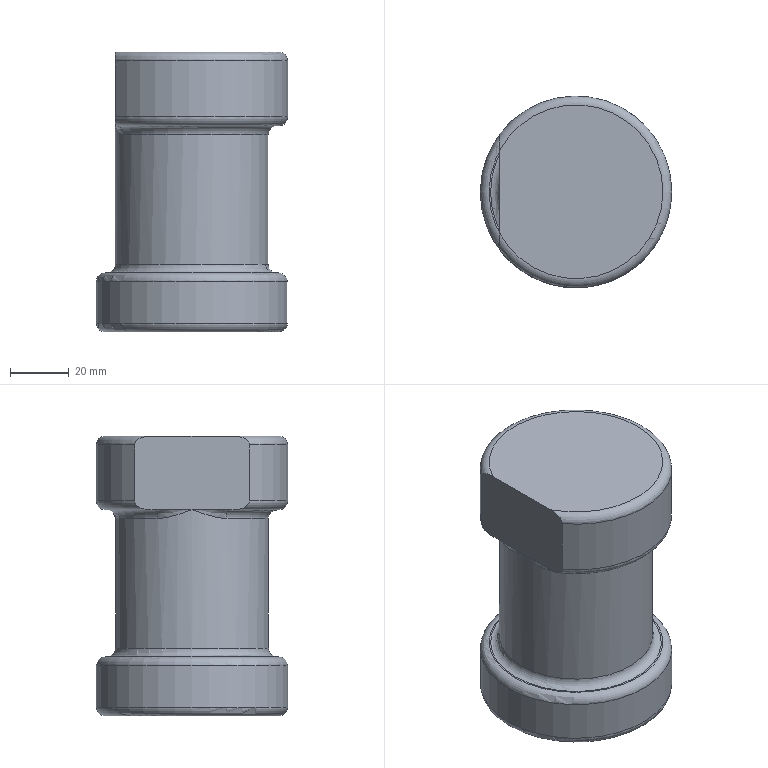Part | NX | features solid 2 | 1 solid | 19 faces | box 65 x 65 x 95 mm | volume 199108 mm3 | torus 6 | plane 5 | cylinder 4 | cone 2 | spline 2 | commonest cylinder face diameters 65 x2 28 x1 52 x1
STEP:
#1=CARTESIAN_POINT('',(-546.,345.5,87.));
#2=VERTEX_POINT('',#1);
#3=CARTESIAN_POINT('',(-546.,345.5,68.));
#4=VERTEX_POINT('',#3);
#5=CARTESIAN_POINT('',(-546.,345.5,90.));
#6=DIRECTION('',(0.,0.,-1.));
#7=VECTOR('',#6,1000.);
#8=LINE('',#5,#7);
#9=EDGE_CURVE('',#2,#4,#8,.T.);
#10=ORIENTED_EDGE('',*,*,#9,.T.);
#11=CARTESIAN_POINT('',(-546.,384.5,68.));
#12=VERTEX_POINT('',#11);
#13=CARTESIAN_POINT('',(-520.,365.,68.));
#14=DIRECTION('',(0.,0.,-1.));
#15=DIRECTION('',(-1.,0.,0.));
#16=AXIS2_PLACEMENT_3D('',#13,#14,#15);
#17=CIRCLE('',#16,32.5);
#18=EDGE_CURVE('',#4,#12,#17,.F.);
#19=ORIENTED_EDGE('',*,*,#18,.T.);
#20=CARTESIAN_POINT('',(-546.,384.5,87.));
#21=VERTEX_POINT('',#20);
#22=CARTESIAN_POINT('',(-546.,384.5,90.));
#23=DIRECTION('',(0.,0.,-1.));
#24=VECTOR('',#23,1000.);
#25=LINE('',#22,#24);
#26=EDGE_CURVE('',#12,#21,#25,.F.);
#27=ORIENTED_EDGE('',*,*,#26,.T.);
#28=CARTESIAN_POINT('',(-520.,365.,87.));
#29=DIRECTION('',(0.,0.,-1.));
#30=DIRECTION('',(-1.,0.,0.));
#31=AXIS2_PLACEMENT_3D('',#28,#29,#30);
#32=CIRCLE('',#31,32.5);
#33=EDGE_CURVE('',#21,#2,#32,.T.);
#34=ORIENTED_EDGE('',*,*,#33,.T.);
#35=EDGE_LOOP('',(#10,#19,#27,#34));
#36=FACE_BOUND('',#35,.T.);
#37=CARTESIAN_POINT('',(-520.,365.,-5.));
#38=DIRECTION('',(0.,0.,1.));
#39=DIRECTION('',(1.,0.,0.));
#40=AXIS2_PLACEMENT_3D('',#37,#38,#39);
#41=CYLINDRICAL_SURFACE('',#40,32.5);
#42=ADVANCED_FACE('',(#36),#41,.T.);
#43=CARTESIAN_POINT('',(-546.,351.063,90.));
#44=VERTEX_POINT('',#43);
#45=CARTESIAN_POINT('',(-546.,378.937,90.));
#46=VERTEX_POINT('',#45);
#47=CARTESIAN_POINT('',(-546.,345.5,90.));
#48=DIRECTION('',(0.,1.,0.));
#49=VECTOR('',#48,1000.);
#50=LINE('',#47,#49);
#51=EDGE_CURVE('',#44,#46,#50,.T.);
#52=ORIENTED_EDGE('',*,*,#51,.F.);
#53=CARTESIAN_POINT('',(-520.,365.,90.));
#54=DIRECTION('',(0.,0.,-1.));
#55=DIRECTION('',(-1.,0.,0.));
#56=AXIS2_PLACEMENT_3D('',#53,#54,#55);
#57=CIRCLE('',#56,29.5);
#58=EDGE_CURVE('',#44,#46,#57,.F.);
#59=ORIENTED_EDGE('',*,*,#58,.T.);
#60=EDGE_LOOP('',(#52,#59));
#61=FACE_BOUND('',#60,.T.);
#62=CARTESIAN_POINT('',(-520.,365.,90.));
#63=DIRECTION('',(0.,0.,-1.));
#64=DIRECTION('',(-1.,0.,0.));
#65=AXIS2_PLACEMENT_3D('',#62,#63,#64);
#66=PLANE('',#65);
#67=ADVANCED_FACE('',(#61),#66,.F.);
#68=CARTESIAN_POINT('',(-546.,351.063,65.));
#69=VERTEX_POINT('',#68);
#70=CARTESIAN_POINT('',(-546.,352.155,65.));
#71=VERTEX_POINT('',#70);
#72=CARTESIAN_POINT('',(-546.,365.,65.));
#73=DIRECTION('',(0.,1.,0.));
#74=VECTOR('',#73,1000.);
#75=LINE('',#72,#74);
#76=EDGE_CURVE('',#69,#71,#75,.T.);
#77=ORIENTED_EDGE('',*,*,#76,.T.);
#78=CARTESIAN_POINT('',(-546.,377.845,65.));
#79=VERTEX_POINT('',#78);
#80=CARTESIAN_POINT('',(-520.,365.,65.));
#81=DIRECTION('',(0.,0.,-1.));
#82=DIRECTION('',(-1.,0.,0.));
#83=AXIS2_PLACEMENT_3D('',#80,#81,#82);
#84=CIRCLE('',#83,29.);
#85=EDGE_CURVE('',#71,#79,#84,.F.);
#86=ORIENTED_EDGE('',*,*,#85,.T.);
#87=CARTESIAN_POINT('',(-546.,378.937,65.));
#88=VERTEX_POINT('',#87);
#89=CARTESIAN_POINT('',(-546.,365.,65.));
#90=DIRECTION('',(0.,1.,0.));
#91=VECTOR('',#90,1000.);
#92=LINE('',#89,#91);
#93=EDGE_CURVE('',#79,#88,#92,.T.);
#94=ORIENTED_EDGE('',*,*,#93,.T.);
#95=CARTESIAN_POINT('',(-520.,365.,65.));
#96=DIRECTION('',(0.,0.,-1.));
#97=DIRECTION('',(-1.,0.,0.));
#98=AXIS2_PLACEMENT_3D('',#95,#96,#97);
#99=CIRCLE('',#98,29.5);
#100=EDGE_CURVE('',#88,#69,#99,.T.);
#101=ORIENTED_EDGE('',*,*,#100,.T.);
#102=EDGE_LOOP('',(#77,#86,#94,#101));
#103=FACE_BOUND('',#102,.T.);
#104=CARTESIAN_POINT('',(-520.,365.,65.));
#105=DIRECTION('',(0.,0.,-1.));
#106=DIRECTION('',(-1.,0.,0.));
#107=AXIS2_PLACEMENT_3D('',#104,#105,#106);
#108=PLANE('',#107);
#109=ADVANCED_FACE('',(#103),#108,.T.);
#110=ORIENTED_EDGE('',*,*,#58,.F.);
#111=CARTESIAN_POINT('',(-546.,351.063,90.));
#112=CARTESIAN_POINT('',(-546.,349.918,90.));
#113=CARTESIAN_POINT('',(-546.,348.171,89.797));
#114=CARTESIAN_POINT('',(-546.,346.107,88.666));
#115=CARTESIAN_POINT('',(-546.,345.5,87.58));
#116=CARTESIAN_POINT('',(-546.,345.5,87.));
#117=B_SPLINE_CURVE_WITH_KNOTS('',3,(#111,#112,#113,#114,#115,#116),.UNSPECIFIED.,.F.,.F.,(4,1,1,4),(0.02888,0.03234,0.03407,0.03579),.UNSPECIFIED.);
#118=EDGE_CURVE('',#44,#2,#117,.T.);
#119=ORIENTED_EDGE('',*,*,#118,.T.);
#120=ORIENTED_EDGE('',*,*,#33,.F.);
#121=CARTESIAN_POINT('',(-546.,384.5,87.));
#122=CARTESIAN_POINT('',(-546.,384.5,87.578));
#123=CARTESIAN_POINT('',(-546.,383.893,88.668));
#124=CARTESIAN_POINT('',(-546.,381.825,89.797));
#125=CARTESIAN_POINT('',(-546.,380.08,90.));
#126=CARTESIAN_POINT('',(-546.,378.937,90.));
#127=B_SPLINE_CURVE_WITH_KNOTS('',3,(#121,#122,#123,#124,#125,#126),.UNSPECIFIED.,.F.,.F.,(4,1,1,4),(0.01647,0.0182,0.01994,0.02342),.UNSPECIFIED.);
#128=EDGE_CURVE('',#21,#46,#127,.T.);
#129=ORIENTED_EDGE('',*,*,#128,.T.);
#130=EDGE_LOOP('',(#110,#119,#120,#129));
#131=FACE_BOUND('',#130,.T.);
#132=CARTESIAN_POINT('',(-520.,365.,87.));
#133=DIRECTION('',(0.,0.,-1.));
#134=DIRECTION('',(-1.,0.,0.));
#135=AXIS2_PLACEMENT_3D('',#132,#133,#134);
#136=TOROIDAL_SURFACE('',#135,29.5,3.);
#137=ADVANCED_FACE('',(#131),#136,.T.);
#138=CARTESIAN_POINT('',(-549.,365.,15.));
#139=VERTEX_POINT('',#138);
#140=CARTESIAN_POINT('',(-520.,365.,15.));
#141=DIRECTION('',(0.,0.,-1.));
#142=DIRECTION('',(-1.,0.,0.));
#143=AXIS2_PLACEMENT_3D('',#140,#141,#142);
#144=CIRCLE('',#143,29.);
#145=EDGE_CURVE('',#139,#139,#144,.T.);
#146=ORIENTED_EDGE('',*,*,#145,.T.);
#147=EDGE_LOOP('',(#146));
#148=FACE_BOUND('',#147,.T.);
#149=CARTESIAN_POINT('',(-549.5,365.,15.));
#150=VERTEX_POINT('',#149);
#151=CARTESIAN_POINT('',(-520.,365.,15.));
#152=DIRECTION('',(0.,0.,-1.));
#153=DIRECTION('',(-1.,0.,0.));
#154=AXIS2_PLACEMENT_3D('',#151,#152,#153);
#155=CIRCLE('',#154,29.5);
#156=EDGE_CURVE('',#150,#150,#155,.F.);
#157=ORIENTED_EDGE('',*,*,#156,.T.);
#158=EDGE_LOOP('',(#157));
#159=FACE_BOUND('',#158,.T.);
#160=CARTESIAN_POINT('',(-520.,365.,15.));
#161=DIRECTION('',(0.,0.,-1.));
#162=DIRECTION('',(-1.,0.,0.));
#163=AXIS2_PLACEMENT_3D('',#160,#161,#162);
#164=PLANE('',#163);
#165=ADVANCED_FACE('',(#148,#159),#164,.F.);
#166=CARTESIAN_POINT('',(-546.,365.,18.));
#167=VERTEX_POINT('',#166);
#168=CARTESIAN_POINT('',(-520.,365.,18.));
#169=DIRECTION('',(0.,0.,-1.));
#170=DIRECTION('',(-1.,0.,0.));
#171=AXIS2_PLACEMENT_3D('',#168,#169,#170);
#172=CIRCLE('',#171,26.);
#173=EDGE_CURVE('',#167,#167,#172,.F.);
#174=ORIENTED_EDGE('',*,*,#173,.T.);
#175=EDGE_LOOP('',(#174));
#176=FACE_BOUND('',#175,.T.);
#177=CARTESIAN_POINT('',(-543.31,353.484,62.));
#178=VERTEX_POINT('',#177);
#179=CARTESIAN_POINT('',(-546.,365.,65.));
#180=VERTEX_POINT('',#179);
#181=CARTESIAN_POINT('',(-543.31,353.484,62.));
#182=CARTESIAN_POINT('',(-544.233,355.351,62.));
#183=CARTESIAN_POINT('',(-545.571,359.193,62.924));
#184=CARTESIAN_POINT('',(-546.,363.039,64.297));
#185=CARTESIAN_POINT('',(-546.,365.,65.));
#186=B_SPLINE_CURVE_WITH_KNOTS('',3,(#181,#182,#183,#184,#185),.UNSPECIFIED.,.F.,.F.,(4,1,4),(0.,0.006249,0.0125),.UNSPECIFIED.);
#187=EDGE_CURVE('',#178,#180,#186,.T.);
#188=ORIENTED_EDGE('',*,*,#187,.T.);
#189=CARTESIAN_POINT('',(-543.31,376.516,62.));
#190=VERTEX_POINT('',#189);
#191=CARTESIAN_POINT('',(-543.31,376.516,62.));
#192=CARTESIAN_POINT('',(-544.233,374.649,62.));
#193=CARTESIAN_POINT('',(-545.571,370.807,62.924));
#194=CARTESIAN_POINT('',(-546.,366.961,64.297));
#195=CARTESIAN_POINT('',(-546.,365.,65.));
#196=B_SPLINE_CURVE_WITH_KNOTS('',3,(#191,#192,#193,#194,#195),.UNSPECIFIED.,.F.,.F.,(4,1,4),(0.,0.006249,0.0125),.UNSPECIFIED.);
#197=EDGE_CURVE('',#180,#190,#196,.F.);
#198=ORIENTED_EDGE('',*,*,#197,.T.);
#199=CARTESIAN_POINT('',(-520.,365.,62.));
#200=DIRECTION('',(0.,0.,-1.));
#201=DIRECTION('',(-1.,0.,0.));
#202=AXIS2_PLACEMENT_3D('',#199,#200,#201);
#203=CIRCLE('',#202,26.);
#204=EDGE_CURVE('',#190,#178,#203,.T.);
#205=ORIENTED_EDGE('',*,*,#204,.T.);
#206=EDGE_LOOP('',(#188,#198,#205));
#207=FACE_BOUND('',#206,.T.);
#208=CARTESIAN_POINT('',(-520.,365.,40.));
#209=DIRECTION('',(0.,0.,-1.));
#210=DIRECTION('',(-1.,0.,0.));
#211=AXIS2_PLACEMENT_3D('',#208,#209,#210);
#212=CYLINDRICAL_SURFACE('',#211,26.);
#213=ADVANCED_FACE('',(#176,#207),#212,.T.);
#214=CARTESIAN_POINT('',(-549.5,365.,-5.));
#215=VERTEX_POINT('',#214);
#216=CARTESIAN_POINT('',(-520.,365.,-5.));
#217=DIRECTION('',(0.,0.,-1.));
#218=DIRECTION('',(-1.,0.,0.));
#219=AXIS2_PLACEMENT_3D('',#216,#217,#218);
#220=CIRCLE('',#219,29.5);
#221=EDGE_CURVE('',#215,#215,#220,.T.);
#222=ORIENTED_EDGE('',*,*,#221,.T.);
#223=EDGE_LOOP('',(#222));
#224=FACE_BOUND('',#223,.T.);
#225=CARTESIAN_POINT('',(-499.,365.,-5.));
#226=VERTEX_POINT('',#225);
#227=CARTESIAN_POINT('',(-520.,365.,-5.));
#228=DIRECTION('',(0.,0.,1.));
#229=DIRECTION('',(1.,0.,0.));
#230=AXIS2_PLACEMENT_3D('',#227,#228,#229);
#231=CIRCLE('',#230,21.);
#232=EDGE_CURVE('',#226,#226,#231,.T.);
#233=ORIENTED_EDGE('',*,*,#232,.T.);
#234=EDGE_LOOP('',(#233));
#235=FACE_BOUND('',#234,.T.);
#236=CARTESIAN_POINT('',(-520.,365.,-5.));
#237=DIRECTION('',(0.,0.,-1.));
#238=DIRECTION('',(-1.,0.,0.));
#239=AXIS2_PLACEMENT_3D('',#236,#237,#238);
#240=PLANE('',#239);
#241=ADVANCED_FACE('',(#224,#235),#240,.T.);
#242=CARTESIAN_POINT('',(-552.5,365.,-2.));
#243=VERTEX_POINT('',#242);
#244=CARTESIAN_POINT('',(-520.,365.,-2.));
#245=DIRECTION('',(0.,0.,-1.));
#246=DIRECTION('',(-1.,0.,0.));
#247=AXIS2_PLACEMENT_3D('',#244,#245,#246);
#248=CIRCLE('',#247,32.5);
#249=EDGE_CURVE('',#243,#243,#248,.F.);
#250=ORIENTED_EDGE('',*,*,#249,.T.);
#251=EDGE_LOOP('',(#250));
#252=FACE_BOUND('',#251,.T.);
#253=CARTESIAN_POINT('',(-552.5,365.,12.));
#254=VERTEX_POINT('',#253);
#255=CARTESIAN_POINT('',(-520.,365.,12.));
#256=DIRECTION('',(0.,0.,-1.));
#257=DIRECTION('',(-1.,0.,0.));
#258=AXIS2_PLACEMENT_3D('',#255,#256,#257);
#259=CIRCLE('',#258,32.5);
#260=EDGE_CURVE('',#254,#254,#259,.T.);
#261=ORIENTED_EDGE('',*,*,#260,.T.);
#262=EDGE_LOOP('',(#261));
#263=FACE_BOUND('',#262,.T.);
#264=CARTESIAN_POINT('',(-520.,365.,-5.));
#265=DIRECTION('',(0.,0.,1.));
#266=DIRECTION('',(1.,0.,0.));
#267=AXIS2_PLACEMENT_3D('',#264,#265,#266);
#268=CYLINDRICAL_SURFACE('',#267,32.5);
#269=ADVANCED_FACE('',(#252,#263),#268,.T.);
#270=CARTESIAN_POINT('',(-506.,365.,70.));
#271=VERTEX_POINT('',#270);
#272=CARTESIAN_POINT('',(-520.,365.,70.));
#273=DIRECTION('',(0.,0.,1.));
#274=DIRECTION('',(1.,0.,0.));
#275=AXIS2_PLACEMENT_3D('',#272,#273,#274);
#276=CIRCLE('',#275,14.);
#277=EDGE_CURVE('',#271,#271,#276,.T.);
#278=ORIENTED_EDGE('',*,*,#277,.F.);
#279=EDGE_LOOP('',(#278));
#280=FACE_BOUND('',#279,.T.);
#281=CARTESIAN_POINT('',(-520.,365.,73.751));
#282=VERTEX_POINT('',#281);
#283=VERTEX_LOOP('',#282);
#284=FACE_BOUND('',#283,.T.);
#285=CARTESIAN_POINT('',(-520.,365.,70.));
#286=DIRECTION('',(0.,0.,-1.));
#287=DIRECTION('',(-1.,0.,0.));
#288=AXIS2_PLACEMENT_3D('',#285,#286,#287);
#289=CONICAL_SURFACE('',#288,14.,1.309);
#290=ADVANCED_FACE('',(#280,#284),#289,.F.);
#291=ORIENTED_EDGE('',*,*,#277,.T.);
#292=EDGE_LOOP('',(#291));
#293=FACE_BOUND('',#292,.T.);
#294=CARTESIAN_POINT('',(-506.,365.,7.124));
#295=VERTEX_POINT('',#294);
#296=CARTESIAN_POINT('',(-520.,365.,7.124));
#297=DIRECTION('',(0.,0.,1.));
#298=DIRECTION('',(1.,0.,0.));
#299=AXIS2_PLACEMENT_3D('',#296,#297,#298);
#300=CIRCLE('',#299,14.);
#301=EDGE_CURVE('',#295,#295,#300,.T.);
#302=ORIENTED_EDGE('',*,*,#301,.F.);
#303=EDGE_LOOP('',(#302));
#304=FACE_BOUND('',#303,.T.);
#305=CARTESIAN_POINT('',(-520.,365.,70.));
#306=DIRECTION('',(0.,0.,1.));
#307=DIRECTION('',(1.,0.,0.));
#308=AXIS2_PLACEMENT_3D('',#305,#306,#307);
#309=CYLINDRICAL_SURFACE('',#308,14.);
#310=ADVANCED_FACE('',(#293,#304),#309,.F.);
#311=ORIENTED_EDGE('',*,*,#301,.T.);
#312=EDGE_LOOP('',(#311));
#313=FACE_BOUND('',#312,.T.);
#314=ORIENTED_EDGE('',*,*,#232,.F.);
#315=EDGE_LOOP('',(#314));
#316=FACE_BOUND('',#315,.T.);
#317=CARTESIAN_POINT('',(-520.,365.,-5.));
#318=DIRECTION('',(0.,0.,-1.));
#319=DIRECTION('',(-1.,0.,0.));
#320=AXIS2_PLACEMENT_3D('',#317,#318,#319);
#321=CONICAL_SURFACE('',#320,21.,0.5236);
#322=ADVANCED_FACE('',(#313,#316),#321,.F.);
#323=ORIENTED_EDGE('',*,*,#76,.F.);
#324=CARTESIAN_POINT('',(-546.,351.063,65.));
#325=CARTESIAN_POINT('',(-546.,349.908,65.));
#326=CARTESIAN_POINT('',(-546.,348.177,65.202));
#327=CARTESIAN_POINT('',(-546.,346.108,66.334));
#328=CARTESIAN_POINT('',(-546.,345.5,67.414));
#329=CARTESIAN_POINT('',(-546.,345.5,68.));
#330=B_SPLINE_CURVE_WITH_KNOTS('',3,(#324,#325,#326,#327,#328,#329),.UNSPECIFIED.,.F.,.F.,(4,1,1,4),(0.,0.003431,0.005146,0.006862),.UNSPECIFIED.);
#331=EDGE_CURVE('',#69,#4,#330,.T.);
#332=ORIENTED_EDGE('',*,*,#331,.T.);
#333=ORIENTED_EDGE('',*,*,#9,.F.);
#334=ORIENTED_EDGE('',*,*,#118,.F.);
#335=ORIENTED_EDGE('',*,*,#51,.T.);
#336=ORIENTED_EDGE('',*,*,#128,.F.);
#337=ORIENTED_EDGE('',*,*,#26,.F.);
#338=CARTESIAN_POINT('',(-546.,384.5,68.));
#339=CARTESIAN_POINT('',(-546.,384.5,67.413));
#340=CARTESIAN_POINT('',(-546.,383.893,66.337));
#341=CARTESIAN_POINT('',(-546.,381.832,65.204));
#342=CARTESIAN_POINT('',(-546.,380.093,65.));
#343=CARTESIAN_POINT('',(-546.,378.937,65.));
#344=B_SPLINE_CURVE_WITH_KNOTS('',3,(#338,#339,#340,#341,#342,#343),.UNSPECIFIED.,.F.,.F.,(4,1,1,4),(0.,0.001726,0.003452,0.006904),.UNSPECIFIED.);
#345=EDGE_CURVE('',#12,#88,#344,.T.);
#346=ORIENTED_EDGE('',*,*,#345,.T.);
#347=ORIENTED_EDGE('',*,*,#93,.F.);
#348=CARTESIAN_POINT('',(-546.,365.,65.));
#349=DIRECTION('',(0.,1.,0.));
#350=VECTOR('',#349,1000.);
#351=LINE('',#348,#350);
#352=EDGE_CURVE('',#180,#79,#351,.T.);
#353=ORIENTED_EDGE('',*,*,#352,.F.);
#354=CARTESIAN_POINT('',(-546.,365.,65.));
#355=DIRECTION('',(0.,1.,0.));
#356=VECTOR('',#355,1000.);
#357=LINE('',#354,#356);
#358=EDGE_CURVE('',#71,#180,#357,.T.);
#359=ORIENTED_EDGE('',*,*,#358,.F.);
#360=EDGE_LOOP('',(#323,#332,#333,#334,#335,#336,#337,#346,#347,#353,#359));
#361=FACE_BOUND('',#360,.T.);
#362=CARTESIAN_POINT('',(-546.,345.5,90.));
#363=DIRECTION('',(-1.,0.,0.));
#364=DIRECTION('',(0.,0.,1.));
#365=AXIS2_PLACEMENT_3D('',#362,#363,#364);
#366=PLANE('',#365);
#367=ADVANCED_FACE('',(#361),#366,.T.);
#368=ORIENTED_EDGE('',*,*,#249,.F.);
#369=EDGE_LOOP('',(#368));
#370=FACE_BOUND('',#369,.T.);
#371=ORIENTED_EDGE('',*,*,#221,.F.);
#372=EDGE_LOOP('',(#371));
#373=FACE_BOUND('',#372,.T.);
#374=CARTESIAN_POINT('',(-520.,365.,-2.));
#375=DIRECTION('',(0.,0.,-1.));
#376=DIRECTION('',(-1.,0.,0.));
#377=AXIS2_PLACEMENT_3D('',#374,#375,#376);
#378=TOROIDAL_SURFACE('',#377,29.5,3.);
#379=ADVANCED_FACE('',(#370,#373),#378,.T.);
#380=ORIENTED_EDGE('',*,*,#358,.T.);
#381=ORIENTED_EDGE('',*,*,#187,.F.);
#382=CARTESIAN_POINT('',(-546.,352.155,62.));
#383=DIRECTION('',(0.4429,-0.8966,0.));
#384=DIRECTION('',(-0.8966,-0.4429,0.));
#385=AXIS2_PLACEMENT_3D('',#382,#383,#384);
#386=CIRCLE('',#385,3.);
#387=EDGE_CURVE('',#71,#178,#386,.F.);
#388=ORIENTED_EDGE('',*,*,#387,.F.);
#389=EDGE_LOOP('',(#380,#381,#388));
#390=FACE_BOUND('',#389,.T.);
#391=CARTESIAN_POINT('',(-543.31,353.484,62.));
#392=CARTESIAN_POINT('',(-543.31,353.484,65.));
#393=CARTESIAN_POINT('',(-546.,352.155,65.));
#394=CARTESIAN_POINT('',(-543.767,354.407,62.));
#395=CARTESIAN_POINT('',(-543.642,354.154,64.576));
#396=CARTESIAN_POINT('',(-546.,353.185,65.));
#397=CARTESIAN_POINT('',(-544.558,356.284,62.245));
#398=CARTESIAN_POINT('',(-544.393,355.827,64.102));
#399=CARTESIAN_POINT('',(-546.,355.278,65.));
#400=CARTESIAN_POINT('',(-545.676,360.138,63.248));
#401=CARTESIAN_POINT('',(-545.587,359.67,64.099));
#402=CARTESIAN_POINT('',(-546.,359.577,65.));
#403=CARTESIAN_POINT('',(-546.,363.037,64.296));
#404=CARTESIAN_POINT('',(-546.,362.924,64.648));
#405=CARTESIAN_POINT('',(-546.,362.811,65.));
#406=CARTESIAN_POINT('',(-546.,365.,65.));
#407=CARTESIAN_POINT('',(-546.,365.,65.));
#408=CARTESIAN_POINT('',(-546.,365.,65.));
#409=(BOUNDED_SURFACE()B_SPLINE_SURFACE(3,2,((#391,#392,#393),(#394,#395,#396),(#397,#398,#399),(#400,#401,#402),(#403,#404,#405),(#406,#407,#408)),.UNSPECIFIED.,.F.,.F.,.F.)B_SPLINE_SURFACE_WITH_KNOTS((4,1,1,4),(3,3),(0.00704,0.01049,0.01394,0.02084),(0.,1.),.UNSPECIFIED.)GEOMETRIC_REPRESENTATION_ITEM()RATIONAL_B_SPLINE_SURFACE(((1.,0.7071,1.),(1.,0.7609,1.),(1.,0.8488,1.),(1.,0.9673,1.),(1.,1.,1.),(1.,1.,1.)))REPRESENTATION_ITEM('')SURFACE());
#410=ADVANCED_FACE('',(#390),#409,.F.);
#411=ORIENTED_EDGE('',*,*,#387,.T.);
#412=ORIENTED_EDGE('',*,*,#204,.F.);
#413=CARTESIAN_POINT('',(-546.,377.845,62.));
#414=DIRECTION('',(0.4429,0.8966,0.));
#415=DIRECTION('',(0.8966,-0.4429,0.));
#416=AXIS2_PLACEMENT_3D('',#413,#414,#415);
#417=CIRCLE('',#416,3.);
#418=EDGE_CURVE('',#79,#190,#417,.T.);
#419=ORIENTED_EDGE('',*,*,#418,.F.);
#420=ORIENTED_EDGE('',*,*,#85,.F.);
#421=EDGE_LOOP('',(#411,#412,#419,#420));
#422=FACE_BOUND('',#421,.T.);
#423=CARTESIAN_POINT('',(-520.,365.,62.));
#424=DIRECTION('',(0.,0.,-1.));
#425=DIRECTION('',(-1.,0.,0.));
#426=AXIS2_PLACEMENT_3D('',#423,#424,#425);
#427=TOROIDAL_SURFACE('',#426,29.,3.);
#428=ADVANCED_FACE('',(#422),#427,.F.);
#429=ORIENTED_EDGE('',*,*,#197,.F.);
#430=ORIENTED_EDGE('',*,*,#352,.T.);
#431=ORIENTED_EDGE('',*,*,#418,.T.);
#432=EDGE_LOOP('',(#429,#430,#431));
#433=FACE_BOUND('',#432,.T.);
#434=CARTESIAN_POINT('',(-546.,377.845,65.));
#435=CARTESIAN_POINT('',(-543.31,376.516,65.));
#436=CARTESIAN_POINT('',(-543.31,376.516,62.));
#437=CARTESIAN_POINT('',(-546.,376.815,65.));
#438=CARTESIAN_POINT('',(-543.642,375.846,64.576));
#439=CARTESIAN_POINT('',(-543.767,375.593,62.));
#440=CARTESIAN_POINT('',(-546.,374.722,65.));
#441=CARTESIAN_POINT('',(-544.393,374.173,64.102));
#442=CARTESIAN_POINT('',(-544.558,373.716,62.245));
#443=CARTESIAN_POINT('',(-546.,370.423,65.));
#444=CARTESIAN_POINT('',(-545.587,370.33,64.099));
#445=CARTESIAN_POINT('',(-545.676,369.862,63.248));
#446=CARTESIAN_POINT('',(-546.,367.189,65.));
#447=CARTESIAN_POINT('',(-546.,367.076,64.648));
#448=CARTESIAN_POINT('',(-546.,366.963,64.296));
#449=CARTESIAN_POINT('',(-546.,365.,65.));
#450=CARTESIAN_POINT('',(-546.,365.,65.));
#451=CARTESIAN_POINT('',(-546.,365.,65.));
#452=(BOUNDED_SURFACE()B_SPLINE_SURFACE(3,2,((#434,#435,#436),(#437,#438,#439),(#440,#441,#442),(#443,#444,#445),(#446,#447,#448),(#449,#450,#451)),.UNSPECIFIED.,.F.,.F.,.F.)B_SPLINE_SURFACE_WITH_KNOTS((4,1,1,4),(3,3),(0.00704,0.01049,0.01394,0.02084),(0.,1.),.UNSPECIFIED.)GEOMETRIC_REPRESENTATION_ITEM()RATIONAL_B_SPLINE_SURFACE(((1.,0.7071,1.),(1.,0.7609,1.),(1.,0.8488,1.),(1.,0.9673,1.),(1.,1.,1.),(1.,1.,1.)))REPRESENTATION_ITEM('')SURFACE());
#453=ADVANCED_FACE('',(#433),#452,.F.);
#454=ORIENTED_EDGE('',*,*,#345,.F.);
#455=ORIENTED_EDGE('',*,*,#18,.F.);
#456=ORIENTED_EDGE('',*,*,#331,.F.);
#457=ORIENTED_EDGE('',*,*,#100,.F.);
#458=EDGE_LOOP('',(#454,#455,#456,#457));
#459=FACE_BOUND('',#458,.T.);
#460=CARTESIAN_POINT('',(-520.,365.,68.));
#461=DIRECTION('',(0.,0.,-1.));
#462=DIRECTION('',(-1.,0.,0.));
#463=AXIS2_PLACEMENT_3D('',#460,#461,#462);
#464=TOROIDAL_SURFACE('',#463,29.5,3.);
#465=ADVANCED_FACE('',(#459),#464,.T.);
#466=ORIENTED_EDGE('',*,*,#173,.F.);
#467=EDGE_LOOP('',(#466));
#468=FACE_BOUND('',#467,.T.);
#469=ORIENTED_EDGE('',*,*,#145,.F.);
#470=EDGE_LOOP('',(#469));
#471=FACE_BOUND('',#470,.T.);
#472=CARTESIAN_POINT('',(-520.,365.,18.));
#473=DIRECTION('',(0.,0.,-1.));
#474=DIRECTION('',(-1.,0.,0.));
#475=AXIS2_PLACEMENT_3D('',#472,#473,#474);
#476=TOROIDAL_SURFACE('',#475,29.,3.);
#477=ADVANCED_FACE('',(#468,#471),#476,.F.);
#478=ORIENTED_EDGE('',*,*,#156,.F.);
#479=EDGE_LOOP('',(#478));
#480=FACE_BOUND('',#479,.T.);
#481=ORIENTED_EDGE('',*,*,#260,.F.);
#482=EDGE_LOOP('',(#481));
#483=FACE_BOUND('',#482,.T.);
#484=CARTESIAN_POINT('',(-520.,365.,12.));
#485=DIRECTION('',(0.,0.,-1.));
#486=DIRECTION('',(-1.,0.,0.));
#487=AXIS2_PLACEMENT_3D('',#484,#485,#486);
#488=TOROIDAL_SURFACE('',#487,29.5,3.);
#489=ADVANCED_FACE('',(#480,#483),#488,.T.);
#490=CLOSED_SHELL('',(#42,#67,#109,#137,#165,#213,#241,#269,#290,#310,#322,#367,#379,#410,#428,#453,#465,#477,#489));
#491=MANIFOLD_SOLID_BREP('',#490);
#492=(LENGTH_UNIT()NAMED_UNIT(*)SI_UNIT(.MILLI.,.METRE.));
#493=UNCERTAINTY_MEASURE_WITH_UNIT(LENGTH_MEASURE(0.0508),#492,'','');
#494=(NAMED_UNIT(*)PLANE_ANGLE_UNIT()SI_UNIT($,.RADIAN.));
#495=(NAMED_UNIT(*)SI_UNIT($,.STERADIAN.)SOLID_ANGLE_UNIT());
#496=(GEOMETRIC_REPRESENTATION_CONTEXT(3)GLOBAL_UNCERTAINTY_ASSIGNED_CONTEXT((#493))GLOBAL_UNIT_ASSIGNED_CONTEXT((#492,#494,#495))REPRESENTATION_CONTEXT('',''));
#497=ADVANCED_BREP_SHAPE_REPRESENTATION('',(#491),#496);